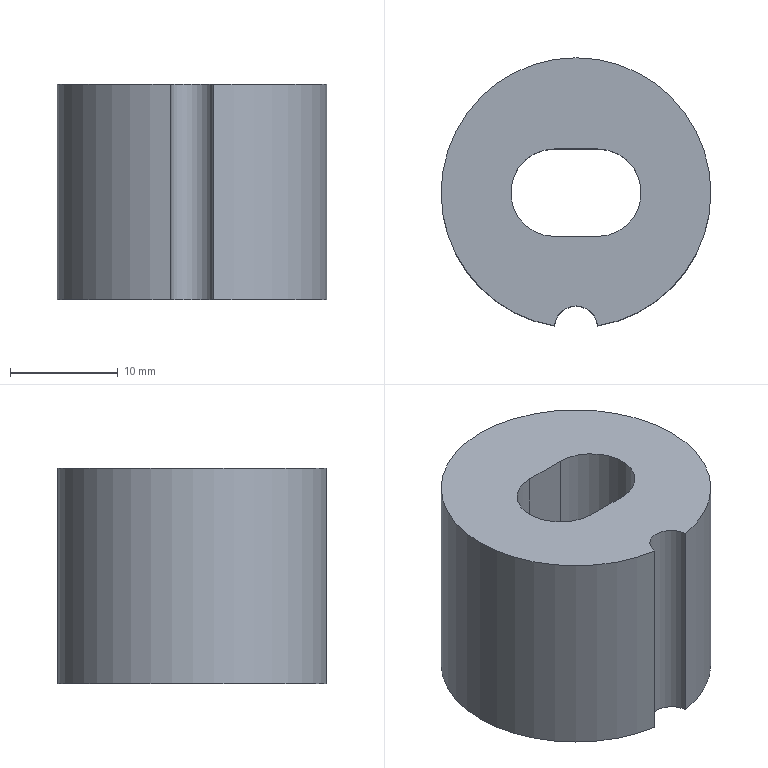Part | NX | features solid 2 | 1 solid | 10 faces | box 25 x 24.84 x 20 mm | volume 6428 mm3 | cylinder 5 | plane 5 | commonest cylinder face diameters 8.1 x2 4 x1 16.6 x1 25 x1
STEP:
#1=CARTESIAN_POINT('',(-1260.42,372.588,38.));
#2=VERTEX_POINT('',#1);
#3=CARTESIAN_POINT('',(-1260.42,372.588,58.));
#4=VERTEX_POINT('',#3);
#5=CARTESIAN_POINT('',(-1260.42,372.588,48.));
#6=DIRECTION('',(0.,0.,1.));
#7=VECTOR('',#6,1000.);
#8=LINE('',#5,#7);
#9=EDGE_CURVE('',#2,#4,#8,.T.);
#10=ORIENTED_EDGE('',*,*,#9,.F.);
#11=CARTESIAN_POINT('',(-1264.407,372.588,38.));
#12=VERTEX_POINT('',#11);
#13=CARTESIAN_POINT('',(-1262.413,384.928,38.));
#14=DIRECTION('',(0.,0.,1.));
#15=DIRECTION('',(0.,-1.,0.));
#16=AXIS2_PLACEMENT_3D('',#13,#14,#15);
#17=CIRCLE('',#16,12.5);
#18=EDGE_CURVE('',#2,#12,#17,.T.);
#19=ORIENTED_EDGE('',*,*,#18,.T.);
#20=CARTESIAN_POINT('',(-1264.407,372.588,58.));
#21=VERTEX_POINT('',#20);
#22=CARTESIAN_POINT('',(-1264.407,372.588,48.));
#23=DIRECTION('',(0.,0.,1.));
#24=VECTOR('',#23,1000.);
#25=LINE('',#22,#24);
#26=EDGE_CURVE('',#21,#12,#25,.F.);
#27=ORIENTED_EDGE('',*,*,#26,.F.);
#28=CARTESIAN_POINT('',(-1262.413,384.928,58.));
#29=DIRECTION('',(0.,0.,1.));
#30=DIRECTION('',(0.,-1.,0.));
#31=AXIS2_PLACEMENT_3D('',#28,#29,#30);
#32=CIRCLE('',#31,12.5);
#33=EDGE_CURVE('',#4,#21,#32,.T.);
#34=ORIENTED_EDGE('',*,*,#33,.F.);
#35=EDGE_LOOP('',(#10,#19,#27,#34));
#36=FACE_BOUND('',#35,.T.);
#37=CARTESIAN_POINT('',(-1262.413,384.928,38.));
#38=DIRECTION('',(0.,0.,1.));
#39=DIRECTION('',(0.,-1.,0.));
#40=AXIS2_PLACEMENT_3D('',#37,#38,#39);
#41=CYLINDRICAL_SURFACE('',#40,12.5);
#42=ADVANCED_FACE('',(#36),#41,.T.);
#43=CARTESIAN_POINT('',(-1262.413,376.628,38.));
#44=VERTEX_POINT('',#43);
#45=CARTESIAN_POINT('',(-1262.413,384.928,38.));
#46=DIRECTION('',(0.,0.,1.));
#47=DIRECTION('',(0.,-1.,0.));
#48=AXIS2_PLACEMENT_3D('',#45,#46,#47);
#49=CIRCLE('',#48,8.3);
#50=EDGE_CURVE('',#44,#44,#49,.T.);
#51=ORIENTED_EDGE('',*,*,#50,.T.);
#52=EDGE_LOOP('',(#51));
#53=FACE_BOUND('',#52,.T.);
#54=ORIENTED_EDGE('',*,*,#18,.F.);
#55=CARTESIAN_POINT('',(-1262.413,372.428,38.));
#56=DIRECTION('',(0.,0.,1.));
#57=DIRECTION('',(0.,-1.,0.));
#58=AXIS2_PLACEMENT_3D('',#55,#56,#57);
#59=CIRCLE('',#58,2.);
#60=EDGE_CURVE('',#2,#12,#59,.T.);
#61=ORIENTED_EDGE('',*,*,#60,.T.);
#62=EDGE_LOOP('',(#54,#61));
#63=FACE_BOUND('',#62,.T.);
#64=CARTESIAN_POINT('',(-1262.413,384.928,38.));
#65=DIRECTION('',(0.,0.,1.));
#66=DIRECTION('',(0.,-1.,0.));
#67=AXIS2_PLACEMENT_3D('',#64,#65,#66);
#68=PLANE('',#67);
#69=ADVANCED_FACE('',(#53,#63),#68,.F.);
#70=CARTESIAN_POINT('',(-1260.413,388.978,58.));
#71=VERTEX_POINT('',#70);
#72=CARTESIAN_POINT('',(-1264.413,388.978,58.));
#73=VERTEX_POINT('',#72);
#74=CARTESIAN_POINT('',(-1260.413,388.978,58.));
#75=DIRECTION('',(-1.,0.,0.));
#76=VECTOR('',#75,1000.);
#77=LINE('',#74,#76);
#78=EDGE_CURVE('',#71,#73,#77,.T.);
#79=ORIENTED_EDGE('',*,*,#78,.F.);
#80=CARTESIAN_POINT('',(-1260.413,380.878,58.));
#81=VERTEX_POINT('',#80);
#82=CARTESIAN_POINT('',(-1260.413,384.928,58.));
#83=DIRECTION('',(0.,0.,1.));
#84=DIRECTION('',(0.,-1.,0.));
#85=AXIS2_PLACEMENT_3D('',#82,#83,#84);
#86=CIRCLE('',#85,4.05);
#87=EDGE_CURVE('',#81,#71,#86,.T.);
#88=ORIENTED_EDGE('',*,*,#87,.F.);
#89=CARTESIAN_POINT('',(-1264.413,380.878,58.));
#90=VERTEX_POINT('',#89);
#91=CARTESIAN_POINT('',(-1260.413,380.878,58.));
#92=DIRECTION('',(-1.,0.,0.));
#93=VECTOR('',#92,1000.);
#94=LINE('',#91,#93);
#95=EDGE_CURVE('',#81,#90,#94,.T.);
#96=ORIENTED_EDGE('',*,*,#95,.T.);
#97=CARTESIAN_POINT('',(-1264.413,384.928,58.));
#98=DIRECTION('',(0.,0.,1.));
#99=DIRECTION('',(0.,-1.,0.));
#100=AXIS2_PLACEMENT_3D('',#97,#98,#99);
#101=CIRCLE('',#100,4.05);
#102=EDGE_CURVE('',#73,#90,#101,.T.);
#103=ORIENTED_EDGE('',*,*,#102,.F.);
#104=EDGE_LOOP('',(#79,#88,#96,#103));
#105=FACE_BOUND('',#104,.T.);
#106=CARTESIAN_POINT('',(-1262.413,372.428,58.));
#107=DIRECTION('',(0.,0.,1.));
#108=DIRECTION('',(0.,-1.,0.));
#109=AXIS2_PLACEMENT_3D('',#106,#107,#108);
#110=CIRCLE('',#109,2.);
#111=EDGE_CURVE('',#4,#21,#110,.T.);
#112=ORIENTED_EDGE('',*,*,#111,.F.);
#113=ORIENTED_EDGE('',*,*,#33,.T.);
#114=EDGE_LOOP('',(#112,#113));
#115=FACE_BOUND('',#114,.T.);
#116=CARTESIAN_POINT('',(-1262.413,384.928,58.));
#117=DIRECTION('',(0.,0.,1.));
#118=DIRECTION('',(0.,-1.,0.));
#119=AXIS2_PLACEMENT_3D('',#116,#117,#118);
#120=PLANE('',#119);
#121=ADVANCED_FACE('',(#105,#115),#120,.T.);
#122=ORIENTED_EDGE('',*,*,#50,.F.);
#123=EDGE_LOOP('',(#122));
#124=FACE_BOUND('',#123,.T.);
#125=CARTESIAN_POINT('',(-1262.413,376.628,50.));
#126=VERTEX_POINT('',#125);
#127=CARTESIAN_POINT('',(-1262.413,384.928,50.));
#128=DIRECTION('',(0.,0.,1.));
#129=DIRECTION('',(0.,-1.,0.));
#130=AXIS2_PLACEMENT_3D('',#127,#128,#129);
#131=CIRCLE('',#130,8.3);
#132=EDGE_CURVE('',#126,#126,#131,.T.);
#133=ORIENTED_EDGE('',*,*,#132,.T.);
#134=EDGE_LOOP('',(#133));
#135=FACE_BOUND('',#134,.T.);
#136=CARTESIAN_POINT('',(-1262.413,384.928,38.));
#137=DIRECTION('',(0.,0.,1.));
#138=DIRECTION('',(0.,-1.,0.));
#139=AXIS2_PLACEMENT_3D('',#136,#137,#138);
#140=CYLINDRICAL_SURFACE('',#139,8.3);
#141=ADVANCED_FACE('',(#124,#135),#140,.F.);
#142=CARTESIAN_POINT('',(-1260.413,380.878,50.));
#143=VERTEX_POINT('',#142);
#144=CARTESIAN_POINT('',(-1260.413,388.978,50.));
#145=VERTEX_POINT('',#144);
#146=CARTESIAN_POINT('',(-1260.413,384.928,50.));
#147=DIRECTION('',(0.,0.,1.));
#148=DIRECTION('',(0.,-1.,0.));
#149=AXIS2_PLACEMENT_3D('',#146,#147,#148);
#150=CIRCLE('',#149,4.05);
#151=EDGE_CURVE('',#143,#145,#150,.T.);
#152=ORIENTED_EDGE('',*,*,#151,.T.);
#153=CARTESIAN_POINT('',(-1264.413,388.978,50.));
#154=VERTEX_POINT('',#153);
#155=CARTESIAN_POINT('',(-1262.413,388.978,50.));
#156=DIRECTION('',(-1.,0.,0.));
#157=VECTOR('',#156,1000.);
#158=LINE('',#155,#157);
#159=EDGE_CURVE('',#145,#154,#158,.T.);
#160=ORIENTED_EDGE('',*,*,#159,.T.);
#161=CARTESIAN_POINT('',(-1264.413,380.878,50.));
#162=VERTEX_POINT('',#161);
#163=CARTESIAN_POINT('',(-1264.413,384.928,50.));
#164=DIRECTION('',(0.,0.,1.));
#165=DIRECTION('',(0.,-1.,0.));
#166=AXIS2_PLACEMENT_3D('',#163,#164,#165);
#167=CIRCLE('',#166,4.05);
#168=EDGE_CURVE('',#154,#162,#167,.T.);
#169=ORIENTED_EDGE('',*,*,#168,.T.);
#170=CARTESIAN_POINT('',(-1262.413,380.878,50.));
#171=DIRECTION('',(-1.,0.,0.));
#172=VECTOR('',#171,1000.);
#173=LINE('',#170,#172);
#174=EDGE_CURVE('',#143,#162,#173,.T.);
#175=ORIENTED_EDGE('',*,*,#174,.F.);
#176=EDGE_LOOP('',(#152,#160,#169,#175));
#177=FACE_BOUND('',#176,.T.);
#178=ORIENTED_EDGE('',*,*,#132,.F.);
#179=EDGE_LOOP('',(#178));
#180=FACE_BOUND('',#179,.T.);
#181=CARTESIAN_POINT('',(-1262.413,384.928,50.));
#182=DIRECTION('',(0.,0.,1.));
#183=DIRECTION('',(0.,-1.,0.));
#184=AXIS2_PLACEMENT_3D('',#181,#182,#183);
#185=PLANE('',#184);
#186=ADVANCED_FACE('',(#177,#180),#185,.F.);
#187=ORIENTED_EDGE('',*,*,#9,.T.);
#188=ORIENTED_EDGE('',*,*,#111,.T.);
#189=ORIENTED_EDGE('',*,*,#26,.T.);
#190=ORIENTED_EDGE('',*,*,#60,.F.);
#191=EDGE_LOOP('',(#187,#188,#189,#190));
#192=FACE_BOUND('',#191,.T.);
#193=CARTESIAN_POINT('',(-1262.413,372.428,38.));
#194=DIRECTION('',(0.,0.,1.));
#195=DIRECTION('',(0.,-1.,0.));
#196=AXIS2_PLACEMENT_3D('',#193,#194,#195);
#197=CYLINDRICAL_SURFACE('',#196,2.);
#198=ADVANCED_FACE('',(#192),#197,.F.);
#199=CARTESIAN_POINT('',(-1260.413,388.978,38.));
#200=DIRECTION('',(0.,0.,1.));
#201=VECTOR('',#200,1000.);
#202=LINE('',#199,#201);
#203=EDGE_CURVE('',#145,#71,#202,.T.);
#204=ORIENTED_EDGE('',*,*,#203,.T.);
#205=ORIENTED_EDGE('',*,*,#78,.T.);
#206=CARTESIAN_POINT('',(-1264.413,388.978,38.));
#207=DIRECTION('',(0.,0.,1.));
#208=VECTOR('',#207,1000.);
#209=LINE('',#206,#208);
#210=EDGE_CURVE('',#154,#73,#209,.T.);
#211=ORIENTED_EDGE('',*,*,#210,.F.);
#212=ORIENTED_EDGE('',*,*,#159,.F.);
#213=EDGE_LOOP('',(#204,#205,#211,#212));
#214=FACE_BOUND('',#213,.T.);
#215=CARTESIAN_POINT('',(-1260.413,388.978,38.));
#216=DIRECTION('',(0.,1.,0.));
#217=DIRECTION('',(0.,0.,1.));
#218=AXIS2_PLACEMENT_3D('',#215,#216,#217);
#219=PLANE('',#218);
#220=ADVANCED_FACE('',(#214),#219,.F.);
#221=ORIENTED_EDGE('',*,*,#210,.T.);
#222=ORIENTED_EDGE('',*,*,#102,.T.);
#223=CARTESIAN_POINT('',(-1264.413,380.878,38.));
#224=DIRECTION('',(0.,0.,1.));
#225=VECTOR('',#224,1000.);
#226=LINE('',#223,#225);
#227=EDGE_CURVE('',#162,#90,#226,.T.);
#228=ORIENTED_EDGE('',*,*,#227,.F.);
#229=ORIENTED_EDGE('',*,*,#168,.F.);
#230=EDGE_LOOP('',(#221,#222,#228,#229));
#231=FACE_BOUND('',#230,.T.);
#232=CARTESIAN_POINT('',(-1264.413,384.928,38.));
#233=DIRECTION('',(0.,0.,1.));
#234=DIRECTION('',(0.,-1.,0.));
#235=AXIS2_PLACEMENT_3D('',#232,#233,#234);
#236=CYLINDRICAL_SURFACE('',#235,4.05);
#237=ADVANCED_FACE('',(#231),#236,.F.);
#238=ORIENTED_EDGE('',*,*,#174,.T.);
#239=ORIENTED_EDGE('',*,*,#227,.T.);
#240=ORIENTED_EDGE('',*,*,#95,.F.);
#241=CARTESIAN_POINT('',(-1260.413,380.878,38.));
#242=DIRECTION('',(0.,0.,1.));
#243=VECTOR('',#242,1000.);
#244=LINE('',#241,#243);
#245=EDGE_CURVE('',#143,#81,#244,.T.);
#246=ORIENTED_EDGE('',*,*,#245,.F.);
#247=EDGE_LOOP('',(#238,#239,#240,#246));
#248=FACE_BOUND('',#247,.T.);
#249=CARTESIAN_POINT('',(-1260.413,380.878,38.));
#250=DIRECTION('',(0.,1.,0.));
#251=DIRECTION('',(0.,0.,1.));
#252=AXIS2_PLACEMENT_3D('',#249,#250,#251);
#253=PLANE('',#252);
#254=ADVANCED_FACE('',(#248),#253,.T.);
#255=ORIENTED_EDGE('',*,*,#245,.T.);
#256=ORIENTED_EDGE('',*,*,#87,.T.);
#257=ORIENTED_EDGE('',*,*,#203,.F.);
#258=ORIENTED_EDGE('',*,*,#151,.F.);
#259=EDGE_LOOP('',(#255,#256,#257,#258));
#260=FACE_BOUND('',#259,.T.);
#261=CARTESIAN_POINT('',(-1260.413,384.928,38.));
#262=DIRECTION('',(0.,0.,1.));
#263=DIRECTION('',(0.,-1.,0.));
#264=AXIS2_PLACEMENT_3D('',#261,#262,#263);
#265=CYLINDRICAL_SURFACE('',#264,4.05);
#266=ADVANCED_FACE('',(#260),#265,.F.);
#267=CLOSED_SHELL('',(#42,#69,#121,#141,#186,#198,#220,#237,#254,#266));
#268=MANIFOLD_SOLID_BREP('',#267);
#269=(LENGTH_UNIT()NAMED_UNIT(*)SI_UNIT(.MILLI.,.METRE.));
#270=UNCERTAINTY_MEASURE_WITH_UNIT(LENGTH_MEASURE(0.00001),#269,'','');
#271=(NAMED_UNIT(*)PLANE_ANGLE_UNIT()SI_UNIT($,.RADIAN.));
#272=(NAMED_UNIT(*)SI_UNIT($,.STERADIAN.)SOLID_ANGLE_UNIT());
#273=(GEOMETRIC_REPRESENTATION_CONTEXT(3)GLOBAL_UNCERTAINTY_ASSIGNED_CONTEXT((#270))GLOBAL_UNIT_ASSIGNED_CONTEXT((#269,#271,#272))REPRESENTATION_CONTEXT('',''));
#274=ADVANCED_BREP_SHAPE_REPRESENTATION('',(#268),#273);